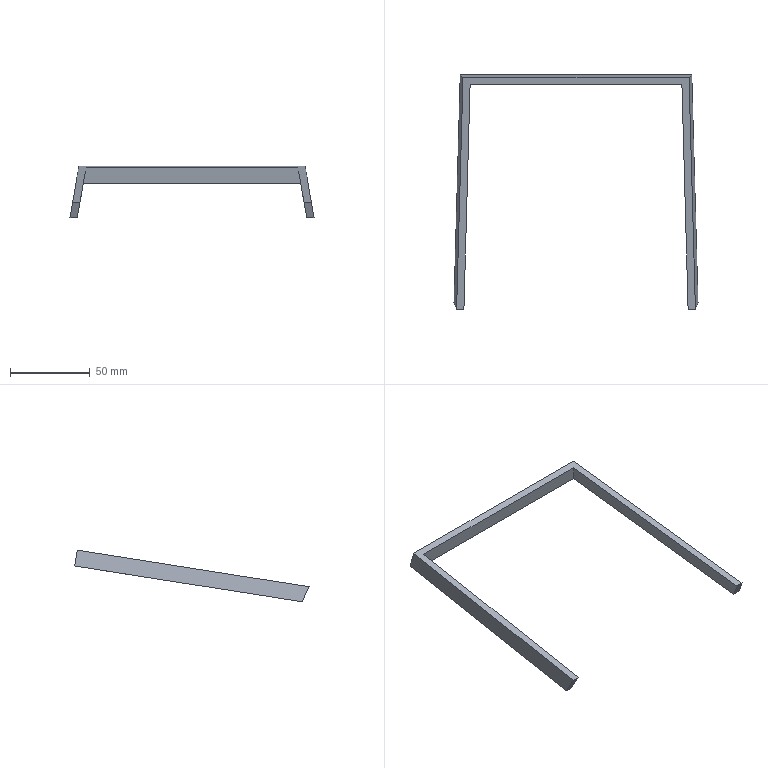Part | STEP file | 1-56.11 | 1 solid | 12 faces | box 152.783 x 146.73 x 32.367 mm | volume 19340 mm3 | plane 12
STEP:
#1=CARTESIAN_POINT('',(0.,0.,0.));
#2=DIRECTION('',(0.,0.,1.));
#3=DIRECTION('',(1.,0.,0.));
#4=AXIS2_PLACEMENT_3D('',#1,#2,#3);
#5=CARTESIAN_POINT('',(-71.823,28.822,-170.894));
#6=VERTEX_POINT('',#5);
#7=CARTESIAN_POINT('',(-76.391,28.822,-170.894));
#8=VERTEX_POINT('',#7);
#9=CARTESIAN_POINT('',(-71.823,28.822,-170.894));
#10=DIRECTION('',(-1.,0.,0.));
#11=VECTOR('',#10,1.);
#12=LINE('',#9,#11);
#13=CARTESIAN_POINT('',(-73.285,26.624,-166.179));
#14=DIRECTION('',(0.,0.9063,0.4226));
#15=DIRECTION('',(0.,0.4226,-0.9063));
#16=AXIS2_PLACEMENT_3D('',#13,#14,#15);
#17=PLANE('',#16);
#18=CARTESIAN_POINT('',(5.202,-1.462));
#19=DIRECTION('',(0.,1.));
#20=VECTOR('',#19,1.);
#21=LINE('',#18,#20);
#22=(GEOMETRIC_REPRESENTATION_CONTEXT(2)PARAMETRIC_REPRESENTATION_CONTEXT()REPRESENTATION_CONTEXT('',''));
#23=DEFINITIONAL_REPRESENTATION('',(#21),#22);
#24=PCURVE('',#17,#23);
#25=CARTESIAN_POINT('',(-72.146,100.013,-159.645));
#26=DIRECTION('',(0.,-0.1561,0.9877));
#27=DIRECTION('',(0.,0.9877,0.1561));
#28=AXIS2_PLACEMENT_3D('',#25,#26,#27);
#29=PLANE('',#28);
#30=CARTESIAN_POINT('',(-72.074,-0.3226));
#31=DIRECTION('',(0.,1.));
#32=VECTOR('',#31,1.);
#33=LINE('',#30,#32);
#34=(GEOMETRIC_REPRESENTATION_CONTEXT(2)PARAMETRIC_REPRESENTATION_CONTEXT()REPRESENTATION_CONTEXT('',''));
#35=DEFINITIONAL_REPRESENTATION('',(#33),#34);
#36=PCURVE('',#29,#35);
#37=SURFACE_CURVE('',#12,(#24,#36),.PCURVE_S1.);
#38=EDGE_CURVE('',#6,#8,#37,.T.);
#39=ORIENTED_EDGE('',*,*,#38,.T.);
#40=CARTESIAN_POINT('',(-74.747,24.425,-161.465));
#41=VERTEX_POINT('',#40);
#42=CARTESIAN_POINT('',(-76.391,28.822,-170.894));
#43=DIRECTION('',(0.1561,-0.4174,0.8952));
#44=VECTOR('',#43,1.);
#45=LINE('',#42,#44);
#46=CARTESIAN_POINT('',(5.202,3.106));
#47=DIRECTION('',(-0.9877,-0.1561));
#48=VECTOR('',#47,1.);
#49=LINE('',#46,#48);
#50=(GEOMETRIC_REPRESENTATION_CONTEXT(2)PARAMETRIC_REPRESENTATION_CONTEXT()REPRESENTATION_CONTEXT('',''));
#51=DEFINITIONAL_REPRESENTATION('',(#49),#50);
#52=PCURVE('',#17,#51);
#53=CARTESIAN_POINT('',(-63.833,90.,-98.893));
#54=DIRECTION('',(-0.9851,0.,0.1718));
#55=DIRECTION('',(0.1718,0.,0.9851));
#56=AXIS2_PLACEMENT_3D('',#53,#54,#55);
#57=PLANE('',#56);
#58=CARTESIAN_POINT('',(-73.088,-61.178));
#59=DIRECTION('',(0.9087,-0.4174));
#60=VECTOR('',#59,1.);
#61=LINE('',#58,#60);
#62=(GEOMETRIC_REPRESENTATION_CONTEXT(2)PARAMETRIC_REPRESENTATION_CONTEXT()REPRESENTATION_CONTEXT('',''));
#63=DEFINITIONAL_REPRESENTATION('',(#61),#62);
#64=PCURVE('',#57,#63);
#65=SURFACE_CURVE('',#45,(#52,#64),.PCURVE_S1.);
#66=EDGE_CURVE('',#8,#41,#65,.T.);
#67=ORIENTED_EDGE('',*,*,#66,.T.);
#68=CARTESIAN_POINT('',(-70.179,24.425,-161.465));
#69=VERTEX_POINT('',#68);
#70=CARTESIAN_POINT('',(-70.179,24.425,-161.465));
#71=DIRECTION('',(-1.,0.,0.));
#72=VECTOR('',#71,1.);
#73=LINE('',#70,#72);
#74=CARTESIAN_POINT('',(-5.202,-3.106));
#75=DIRECTION('',(0.,1.));
#76=VECTOR('',#75,1.);
#77=LINE('',#74,#76);
#78=(GEOMETRIC_REPRESENTATION_CONTEXT(2)PARAMETRIC_REPRESENTATION_CONTEXT()REPRESENTATION_CONTEXT('',''));
#79=DEFINITIONAL_REPRESENTATION('',(#77),#78);
#80=PCURVE('',#17,#79);
#81=CARTESIAN_POINT('',(-80.434,-353.244,-221.14));
#82=DIRECTION('',(0.,0.1561,-0.9877));
#83=DIRECTION('',(0.,-0.9877,-0.1561));
#84=AXIS2_PLACEMENT_3D('',#81,#82,#83);
#85=PLANE('',#84);
#86=CARTESIAN_POINT('',(-382.355,-10.256));
#87=DIRECTION('',(0.,1.));
#88=VECTOR('',#87,1.);
#89=LINE('',#86,#88);
#90=(GEOMETRIC_REPRESENTATION_CONTEXT(2)PARAMETRIC_REPRESENTATION_CONTEXT()REPRESENTATION_CONTEXT('',''));
#91=DEFINITIONAL_REPRESENTATION('',(#89),#90);
#92=PCURVE('',#85,#91);
#93=SURFACE_CURVE('',#73,(#80,#92),.PCURVE_S1.);
#94=EDGE_CURVE('',#69,#41,#93,.T.);
#95=ORIENTED_EDGE('',*,*,#94,.F.);
#96=CARTESIAN_POINT('',(-70.179,24.425,-161.465));
#97=DIRECTION('',(-0.1561,0.4174,-0.8952));
#98=VECTOR('',#97,1.);
#99=LINE('',#96,#98);
#100=CARTESIAN_POINT('',(-5.202,-3.106));
#101=DIRECTION('',(0.9877,0.1561));
#102=VECTOR('',#101,1.);
#103=LINE('',#100,#102);
#104=(GEOMETRIC_REPRESENTATION_CONTEXT(2)PARAMETRIC_REPRESENTATION_CONTEXT()REPRESENTATION_CONTEXT('',''));
#105=DEFINITIONAL_REPRESENTATION('',(#103),#104);
#106=PCURVE('',#17,#105);
#107=CARTESIAN_POINT('',(-59.4,90.,-99.667));
#108=DIRECTION('',(0.9851,0.,-0.1718));
#109=DIRECTION('',(-0.1718,0.,-0.9851));
#110=AXIS2_PLACEMENT_3D('',#107,#108,#109);
#111=PLANE('',#110);
#112=CARTESIAN_POINT('',(62.731,-65.575));
#113=DIRECTION('',(0.9087,0.4174));
#114=VECTOR('',#113,1.);
#115=LINE('',#112,#114);
#116=(GEOMETRIC_REPRESENTATION_CONTEXT(2)PARAMETRIC_REPRESENTATION_CONTEXT()REPRESENTATION_CONTEXT('',''));
#117=DEFINITIONAL_REPRESENTATION('',(#115),#116);
#118=PCURVE('',#111,#117);
#119=SURFACE_CURVE('',#99,(#106,#118),.PCURVE_S1.);
#120=EDGE_CURVE('',#69,#6,#119,.T.);
#121=ORIENTED_EDGE('',*,*,#120,.T.);
#122=EDGE_LOOP('',(#39,#67,#95,#121));
#123=FACE_BOUND('',#122,.F.);
#124=ADVANCED_FACE('',(#123),#17,.F.);
#125=ORIENTED_EDGE('',*,*,#120,.T.);
#126=CARTESIAN_POINT('',(-68.023,166.711,-149.107));
#127=VERTEX_POINT('',#126);
#128=CARTESIAN_POINT('',(-71.823,28.822,-170.894));
#129=DIRECTION('',(0.02721,0.9874,0.156));
#130=VECTOR('',#129,1.);
#131=LINE('',#128,#130);
#132=CARTESIAN_POINT('',(72.303,-61.178));
#133=DIRECTION('',(-0.1584,0.9874));
#134=VECTOR('',#133,1.);
#135=LINE('',#132,#134);
#136=(GEOMETRIC_REPRESENTATION_CONTEXT(2)PARAMETRIC_REPRESENTATION_CONTEXT()REPRESENTATION_CONTEXT('',''));
#137=DEFINITIONAL_REPRESENTATION('',(#135),#136);
#138=PCURVE('',#111,#137);
#139=CARTESIAN_POINT('',(-72.074,-0.3226));
#140=DIRECTION('',(0.9996,-0.02721));
#141=VECTOR('',#140,1.);
#142=LINE('',#139,#141);
#143=(GEOMETRIC_REPRESENTATION_CONTEXT(2)PARAMETRIC_REPRESENTATION_CONTEXT()REPRESENTATION_CONTEXT('',''));
#144=DEFINITIONAL_REPRESENTATION('',(#142),#143);
#145=PCURVE('',#29,#144);
#146=SURFACE_CURVE('',#131,(#138,#145),.PCURVE_S1.);
#147=EDGE_CURVE('',#6,#127,#146,.T.);
#148=ORIENTED_EDGE('',*,*,#147,.T.);
#149=CARTESIAN_POINT('',(-66.301,165.146,-139.231));
#150=VERTEX_POINT('',#149);
#151=CARTESIAN_POINT('',(-66.301,165.146,-139.231));
#152=DIRECTION('',(-0.1698,0.1542,-0.9733));
#153=VECTOR('',#152,1.);
#154=LINE('',#151,#153);
#155=CARTESIAN_POINT('',(40.162,75.146));
#156=DIRECTION('',(0.988,0.1542));
#157=VECTOR('',#156,1.);
#158=LINE('',#155,#157);
#159=(GEOMETRIC_REPRESENTATION_CONTEXT(2)PARAMETRIC_REPRESENTATION_CONTEXT()REPRESENTATION_CONTEXT('',''));
#160=DEFINITIONAL_REPRESENTATION('',(#158),#159);
#161=PCURVE('',#111,#160);
#162=CARTESIAN_POINT('',(0.,165.928,-144.17));
#163=DIRECTION('',(0.,0.9877,0.1565));
#164=DIRECTION('',(0.,0.1565,-0.9877));
#165=AXIS2_PLACEMENT_3D('',#162,#163,#164);
#166=PLANE('',#165);
#167=CARTESIAN_POINT('',(-5.,66.301));
#168=DIRECTION('',(0.9855,0.1698));
#169=VECTOR('',#168,1.);
#170=LINE('',#167,#169);
#171=(GEOMETRIC_REPRESENTATION_CONTEXT(2)PARAMETRIC_REPRESENTATION_CONTEXT()REPRESENTATION_CONTEXT('',''));
#172=DEFINITIONAL_REPRESENTATION('',(#170),#171);
#173=PCURVE('',#166,#172);
#174=SURFACE_CURVE('',#154,(#161,#173),.PCURVE_S1.);
#175=EDGE_CURVE('',#150,#127,#174,.T.);
#176=ORIENTED_EDGE('',*,*,#175,.F.);
#177=CARTESIAN_POINT('',(-66.3,165.146,-139.23));
#178=DIRECTION('',(-0.02721,-0.9874,-0.156));
#179=VECTOR('',#178,1.);
#180=LINE('',#177,#179);
#181=CARTESIAN_POINT('',(40.16,75.146));
#182=DIRECTION('',(0.1584,-0.9874));
#183=VECTOR('',#182,1.);
#184=LINE('',#181,#183);
#185=(GEOMETRIC_REPRESENTATION_CONTEXT(2)PARAMETRIC_REPRESENTATION_CONTEXT()REPRESENTATION_CONTEXT('',''));
#186=DEFINITIONAL_REPRESENTATION('',(#184),#185);
#187=PCURVE('',#111,#186);
#188=CARTESIAN_POINT('',(-524.821,-14.134));
#189=DIRECTION('',(0.9996,0.02721));
#190=VECTOR('',#189,1.);
#191=LINE('',#188,#190);
#192=(GEOMETRIC_REPRESENTATION_CONTEXT(2)PARAMETRIC_REPRESENTATION_CONTEXT()REPRESENTATION_CONTEXT('',''));
#193=DEFINITIONAL_REPRESENTATION('',(#191),#192);
#194=PCURVE('',#85,#193);
#195=SURFACE_CURVE('',#180,(#187,#194),.PCURVE_S1.);
#196=EDGE_CURVE('',#150,#69,#195,.T.);
#197=ORIENTED_EDGE('',*,*,#196,.T.);
#198=EDGE_LOOP('',(#125,#148,#176,#197));
#199=FACE_BOUND('',#198,.T.);
#200=ADVANCED_FACE('',(#199),#111,.T.);
#201=ORIENTED_EDGE('',*,*,#175,.F.);
#202=CARTESIAN_POINT('',(66.301,165.146,-139.231));
#203=VERTEX_POINT('',#202);
#204=CARTESIAN_POINT('',(66.301,165.146,-139.231));
#205=DIRECTION('',(-1.,0.,0.));
#206=VECTOR('',#205,1.);
#207=LINE('',#204,#206);
#208=CARTESIAN_POINT('',(-5.,-66.301));
#209=DIRECTION('',(0.,1.));
#210=VECTOR('',#209,1.);
#211=LINE('',#208,#210);
#212=(GEOMETRIC_REPRESENTATION_CONTEXT(2)PARAMETRIC_REPRESENTATION_CONTEXT()REPRESENTATION_CONTEXT('',''));
#213=DEFINITIONAL_REPRESENTATION('',(#211),#212);
#214=PCURVE('',#166,#213);
#215=CARTESIAN_POINT('',(-524.822,-146.735));
#216=DIRECTION('',(0.,1.));
#217=VECTOR('',#216,1.);
#218=LINE('',#215,#217);
#219=(GEOMETRIC_REPRESENTATION_CONTEXT(2)PARAMETRIC_REPRESENTATION_CONTEXT()REPRESENTATION_CONTEXT('',''));
#220=DEFINITIONAL_REPRESENTATION('',(#218),#219);
#221=PCURVE('',#85,#220);
#222=SURFACE_CURVE('',#207,(#214,#221),.PCURVE_S1.);
#223=EDGE_CURVE('',#203,#150,#222,.T.);
#224=ORIENTED_EDGE('',*,*,#223,.F.);
#225=CARTESIAN_POINT('',(68.023,166.711,-149.107));
#226=VERTEX_POINT('',#225);
#227=CARTESIAN_POINT('',(66.301,165.146,-139.231));
#228=DIRECTION('',(0.1698,0.1542,-0.9733));
#229=VECTOR('',#228,1.);
#230=LINE('',#227,#229);
#231=CARTESIAN_POINT('',(-5.,-66.301));
#232=DIRECTION('',(0.9855,-0.1698));
#233=VECTOR('',#232,1.);
#234=LINE('',#231,#233);
#235=(GEOMETRIC_REPRESENTATION_CONTEXT(2)PARAMETRIC_REPRESENTATION_CONTEXT()REPRESENTATION_CONTEXT('',''));
#236=DEFINITIONAL_REPRESENTATION('',(#234),#235);
#237=PCURVE('',#166,#236);
#238=CARTESIAN_POINT('',(59.4,90.,-99.667));
#239=DIRECTION('',(-0.9851,0.,-0.1718));
#240=DIRECTION('',(-0.1718,0.,0.9851));
#241=AXIS2_PLACEMENT_3D('',#238,#239,#240);
#242=PLANE('',#241);
#243=CARTESIAN_POINT('',(-40.162,75.146));
#244=DIRECTION('',(-0.988,0.1542));
#245=VECTOR('',#244,1.);
#246=LINE('',#243,#245);
#247=(GEOMETRIC_REPRESENTATION_CONTEXT(2)PARAMETRIC_REPRESENTATION_CONTEXT()REPRESENTATION_CONTEXT('',''));
#248=DEFINITIONAL_REPRESENTATION('',(#246),#247);
#249=PCURVE('',#242,#248);
#250=SURFACE_CURVE('',#230,(#237,#249),.PCURVE_S1.);
#251=EDGE_CURVE('',#203,#226,#250,.T.);
#252=ORIENTED_EDGE('',*,*,#251,.T.);
#253=CARTESIAN_POINT('',(68.023,166.711,-149.108));
#254=DIRECTION('',(-1.,0.,0.));
#255=VECTOR('',#254,1.);
#256=LINE('',#253,#255);
#257=CARTESIAN_POINT('',(5.,-68.023));
#258=DIRECTION('',(0.,1.));
#259=VECTOR('',#258,1.);
#260=LINE('',#257,#259);
#261=(GEOMETRIC_REPRESENTATION_CONTEXT(2)PARAMETRIC_REPRESENTATION_CONTEXT()REPRESENTATION_CONTEXT('',''));
#262=DEFINITIONAL_REPRESENTATION('',(#260),#261);
#263=PCURVE('',#166,#262);
#264=CARTESIAN_POINT('',(43.297,126.169,-155.531));
#265=DIRECTION('',(0.,-0.1565,0.9877));
#266=DIRECTION('',(0.,0.9877,0.1565));
#267=AXIS2_PLACEMENT_3D('',#264,#265,#266);
#268=PLANE('',#267);
#269=CARTESIAN_POINT('',(41.047,-24.726));
#270=DIRECTION('',(0.,1.));
#271=VECTOR('',#270,1.);
#272=LINE('',#269,#271);
#273=(GEOMETRIC_REPRESENTATION_CONTEXT(2)PARAMETRIC_REPRESENTATION_CONTEXT()REPRESENTATION_CONTEXT('',''));
#274=DEFINITIONAL_REPRESENTATION('',(#272),#273);
#275=PCURVE('',#268,#274);
#276=SURFACE_CURVE('',#256,(#263,#275),.PCURVE_S1.);
#277=EDGE_CURVE('',#226,#127,#276,.T.);
#278=ORIENTED_EDGE('',*,*,#277,.T.);
#279=EDGE_LOOP('',(#201,#224,#252,#278));
#280=FACE_BOUND('',#279,.F.);
#281=ADVANCED_FACE('',(#280),#166,.F.);
#282=CARTESIAN_POINT('',(71.823,28.822,-170.894));
#283=VERTEX_POINT('',#282);
#284=CARTESIAN_POINT('',(70.179,24.425,-161.465));
#285=VERTEX_POINT('',#284);
#286=CARTESIAN_POINT('',(71.823,28.822,-170.894));
#287=DIRECTION('',(-0.1561,-0.4174,0.8952));
#288=VECTOR('',#287,1.);
#289=LINE('',#286,#288);
#290=CARTESIAN_POINT('',(-72.303,-61.178));
#291=DIRECTION('',(0.9087,-0.4174));
#292=VECTOR('',#291,1.);
#293=LINE('',#290,#292);
#294=(GEOMETRIC_REPRESENTATION_CONTEXT(2)PARAMETRIC_REPRESENTATION_CONTEXT()REPRESENTATION_CONTEXT('',''));
#295=DEFINITIONAL_REPRESENTATION('',(#293),#294);
#296=PCURVE('',#242,#295);
#297=CARTESIAN_POINT('',(73.285,26.624,-166.179));
#298=DIRECTION('',(0.,0.9063,0.4226));
#299=DIRECTION('',(0.,0.4226,-0.9063));
#300=AXIS2_PLACEMENT_3D('',#297,#298,#299);
#301=PLANE('',#300);
#302=CARTESIAN_POINT('',(5.202,1.462));
#303=DIRECTION('',(-0.9877,0.1561));
#304=VECTOR('',#303,1.);
#305=LINE('',#302,#304);
#306=(GEOMETRIC_REPRESENTATION_CONTEXT(2)PARAMETRIC_REPRESENTATION_CONTEXT()REPRESENTATION_CONTEXT('',''));
#307=DEFINITIONAL_REPRESENTATION('',(#305),#306);
#308=PCURVE('',#301,#307);
#309=SURFACE_CURVE('',#289,(#296,#308),.PCURVE_S1.);
#310=EDGE_CURVE('',#283,#285,#309,.T.);
#311=ORIENTED_EDGE('',*,*,#310,.T.);
#312=CARTESIAN_POINT('',(70.179,24.425,-161.465));
#313=DIRECTION('',(-0.02721,0.9874,0.156));
#314=VECTOR('',#313,1.);
#315=LINE('',#312,#314);
#316=CARTESIAN_POINT('',(-62.731,-65.575));
#317=DIRECTION('',(0.1584,0.9874));
#318=VECTOR('',#317,1.);
#319=LINE('',#316,#318);
#320=(GEOMETRIC_REPRESENTATION_CONTEXT(2)PARAMETRIC_REPRESENTATION_CONTEXT()REPRESENTATION_CONTEXT('',''));
#321=DEFINITIONAL_REPRESENTATION('',(#319),#320);
#322=PCURVE('',#242,#321);
#323=CARTESIAN_POINT('',(-382.355,-150.613));
#324=DIRECTION('',(-0.9996,0.02721));
#325=VECTOR('',#324,1.);
#326=LINE('',#323,#325);
#327=(GEOMETRIC_REPRESENTATION_CONTEXT(2)PARAMETRIC_REPRESENTATION_CONTEXT()REPRESENTATION_CONTEXT('',''));
#328=DEFINITIONAL_REPRESENTATION('',(#326),#327);
#329=PCURVE('',#85,#328);
#330=SURFACE_CURVE('',#315,(#322,#329),.PCURVE_S1.);
#331=EDGE_CURVE('',#285,#203,#330,.T.);
#332=ORIENTED_EDGE('',*,*,#331,.T.);
#333=ORIENTED_EDGE('',*,*,#251,.T.);
#334=CARTESIAN_POINT('',(68.023,166.711,-149.106));
#335=DIRECTION('',(0.02721,-0.9874,-0.156));
#336=VECTOR('',#335,1.);
#337=LINE('',#334,#336);
#338=CARTESIAN_POINT('',(-50.186,76.711));
#339=DIRECTION('',(-0.1584,-0.9874));
#340=VECTOR('',#339,1.);
#341=LINE('',#338,#340);
#342=(GEOMETRIC_REPRESENTATION_CONTEXT(2)PARAMETRIC_REPRESENTATION_CONTEXT()REPRESENTATION_CONTEXT('',''));
#343=DEFINITIONAL_REPRESENTATION('',(#341),#342);
#344=PCURVE('',#242,#343);
#345=CARTESIAN_POINT('',(72.146,99.989,-159.649));
#346=DIRECTION('',(0.,-0.1561,0.9877));
#347=DIRECTION('',(0.,0.9877,0.1561));
#348=AXIS2_PLACEMENT_3D('',#345,#346,#347);
#349=PLANE('',#348);
#350=CARTESIAN_POINT('',(67.549,4.123));
#351=DIRECTION('',(-0.9996,-0.02721));
#352=VECTOR('',#351,1.);
#353=LINE('',#350,#352);
#354=(GEOMETRIC_REPRESENTATION_CONTEXT(2)PARAMETRIC_REPRESENTATION_CONTEXT()REPRESENTATION_CONTEXT('',''));
#355=DEFINITIONAL_REPRESENTATION('',(#353),#354);
#356=PCURVE('',#349,#355);
#357=SURFACE_CURVE('',#337,(#344,#356),.PCURVE_S1.);
#358=EDGE_CURVE('',#226,#283,#357,.T.);
#359=ORIENTED_EDGE('',*,*,#358,.T.);
#360=EDGE_LOOP('',(#311,#332,#333,#359));
#361=FACE_BOUND('',#360,.T.);
#362=ADVANCED_FACE('',(#361),#242,.T.);
#363=CARTESIAN_POINT('',(76.391,28.822,-170.894));
#364=VERTEX_POINT('',#363);
#365=CARTESIAN_POINT('',(76.391,28.822,-170.894));
#366=DIRECTION('',(-1.,0.,0.));
#367=VECTOR('',#366,1.);
#368=LINE('',#365,#367);
#369=CARTESIAN_POINT('',(-72.05,-4.245));
#370=DIRECTION('',(0.,1.));
#371=VECTOR('',#370,1.);
#372=LINE('',#369,#371);
#373=(GEOMETRIC_REPRESENTATION_CONTEXT(2)PARAMETRIC_REPRESENTATION_CONTEXT()REPRESENTATION_CONTEXT('',''));
#374=DEFINITIONAL_REPRESENTATION('',(#372),#373);
#375=PCURVE('',#349,#374);
#376=CARTESIAN_POINT('',(5.202,-3.106));
#377=DIRECTION('',(0.,1.));
#378=VECTOR('',#377,1.);
#379=LINE('',#376,#378);
#380=(GEOMETRIC_REPRESENTATION_CONTEXT(2)PARAMETRIC_REPRESENTATION_CONTEXT()REPRESENTATION_CONTEXT('',''));
#381=DEFINITIONAL_REPRESENTATION('',(#379),#380);
#382=PCURVE('',#301,#381);
#383=SURFACE_CURVE('',#368,(#375,#382),.PCURVE_S1.);
#384=EDGE_CURVE('',#364,#283,#383,.T.);
#385=ORIENTED_EDGE('',*,*,#384,.F.);
#386=CARTESIAN_POINT('',(72.591,166.711,-149.107));
#387=VERTEX_POINT('',#386);
#388=CARTESIAN_POINT('',(76.391,28.822,-170.894));
#389=DIRECTION('',(-0.02721,0.9874,0.156));
#390=VECTOR('',#389,1.);
#391=LINE('',#388,#390);
#392=CARTESIAN_POINT('',(-72.05,-4.245));
#393=DIRECTION('',(0.9996,0.02721));
#394=VECTOR('',#393,1.);
#395=LINE('',#392,#394);
#396=(GEOMETRIC_REPRESENTATION_CONTEXT(2)PARAMETRIC_REPRESENTATION_CONTEXT()REPRESENTATION_CONTEXT('',''));
#397=DEFINITIONAL_REPRESENTATION('',(#395),#396);
#398=PCURVE('',#349,#397);
#399=CARTESIAN_POINT('',(63.833,90.,-98.893));
#400=DIRECTION('',(0.9851,0.,0.1718));
#401=DIRECTION('',(0.1718,0.,-0.9851));
#402=AXIS2_PLACEMENT_3D('',#399,#400,#401);
#403=PLANE('',#402);
#404=CARTESIAN_POINT('',(73.088,-61.178));
#405=DIRECTION('',(-0.1584,0.9874));
#406=VECTOR('',#405,1.);
#407=LINE('',#404,#406);
#408=(GEOMETRIC_REPRESENTATION_CONTEXT(2)PARAMETRIC_REPRESENTATION_CONTEXT()REPRESENTATION_CONTEXT('',''));
#409=DEFINITIONAL_REPRESENTATION('',(#407),#408);
#410=PCURVE('',#403,#409);
#411=SURFACE_CURVE('',#391,(#398,#410),.PCURVE_S1.);
#412=EDGE_CURVE('',#364,#387,#411,.T.);
#413=ORIENTED_EDGE('',*,*,#412,.T.);
#414=CARTESIAN_POINT('',(72.591,166.711,-149.108));
#415=DIRECTION('',(-1.,0.,0.));
#416=VECTOR('',#415,1.);
#417=LINE('',#414,#416);
#418=CARTESIAN_POINT('',(67.55,-0.4453));
#419=DIRECTION('',(0.,1.));
#420=VECTOR('',#419,1.);
#421=LINE('',#418,#420);
#422=(GEOMETRIC_REPRESENTATION_CONTEXT(2)PARAMETRIC_REPRESENTATION_CONTEXT()REPRESENTATION_CONTEXT('',''));
#423=DEFINITIONAL_REPRESENTATION('',(#421),#422);
#424=PCURVE('',#349,#423);
#425=CARTESIAN_POINT('',(41.047,-29.294));
#426=DIRECTION('',(0.,1.));
#427=VECTOR('',#426,1.);
#428=LINE('',#425,#427);
#429=(GEOMETRIC_REPRESENTATION_CONTEXT(2)PARAMETRIC_REPRESENTATION_CONTEXT()REPRESENTATION_CONTEXT('',''));
#430=DEFINITIONAL_REPRESENTATION('',(#428),#429);
#431=PCURVE('',#268,#430);
#432=SURFACE_CURVE('',#417,(#424,#431),.PCURVE_S1.);
#433=EDGE_CURVE('',#387,#226,#432,.T.);
#434=ORIENTED_EDGE('',*,*,#433,.T.);
#435=ORIENTED_EDGE('',*,*,#358,.T.);
#436=EDGE_LOOP('',(#385,#413,#434,#435));
#437=FACE_BOUND('',#436,.F.);
#438=ADVANCED_FACE('',(#437),#349,.F.);
#439=ORIENTED_EDGE('',*,*,#384,.T.);
#440=ORIENTED_EDGE('',*,*,#310,.T.);
#441=CARTESIAN_POINT('',(74.747,24.425,-161.465));
#442=VERTEX_POINT('',#441);
#443=CARTESIAN_POINT('',(74.747,24.425,-161.465));
#444=DIRECTION('',(-1.,0.,0.));
#445=VECTOR('',#444,1.);
#446=LINE('',#443,#445);
#447=CARTESIAN_POINT('',(-5.202,-1.462));
#448=DIRECTION('',(0.,1.));
#449=VECTOR('',#448,1.);
#450=LINE('',#447,#449);
#451=(GEOMETRIC_REPRESENTATION_CONTEXT(2)PARAMETRIC_REPRESENTATION_CONTEXT()REPRESENTATION_CONTEXT('',''));
#452=DEFINITIONAL_REPRESENTATION('',(#450),#451);
#453=PCURVE('',#301,#452);
#454=CARTESIAN_POINT('',(-382.355,-155.181));
#455=DIRECTION('',(0.,1.));
#456=VECTOR('',#455,1.);
#457=LINE('',#454,#456);
#458=(GEOMETRIC_REPRESENTATION_CONTEXT(2)PARAMETRIC_REPRESENTATION_CONTEXT()REPRESENTATION_CONTEXT('',''));
#459=DEFINITIONAL_REPRESENTATION('',(#457),#458);
#460=PCURVE('',#85,#459);
#461=SURFACE_CURVE('',#446,(#453,#460),.PCURVE_S1.);
#462=EDGE_CURVE('',#442,#285,#461,.T.);
#463=ORIENTED_EDGE('',*,*,#462,.F.);
#464=CARTESIAN_POINT('',(74.747,24.425,-161.465));
#465=DIRECTION('',(0.1561,0.4174,-0.8952));
#466=VECTOR('',#465,1.);
#467=LINE('',#464,#466);
#468=CARTESIAN_POINT('',(-5.202,-1.462));
#469=DIRECTION('',(0.9877,-0.1561));
#470=VECTOR('',#469,1.);
#471=LINE('',#468,#470);
#472=(GEOMETRIC_REPRESENTATION_CONTEXT(2)PARAMETRIC_REPRESENTATION_CONTEXT()REPRESENTATION_CONTEXT('',''));
#473=DEFINITIONAL_REPRESENTATION('',(#471),#472);
#474=PCURVE('',#301,#473);
#475=CARTESIAN_POINT('',(63.516,-65.575));
#476=DIRECTION('',(0.9087,0.4174));
#477=VECTOR('',#476,1.);
#478=LINE('',#475,#477);
#479=(GEOMETRIC_REPRESENTATION_CONTEXT(2)PARAMETRIC_REPRESENTATION_CONTEXT()REPRESENTATION_CONTEXT('',''));
#480=DEFINITIONAL_REPRESENTATION('',(#478),#479);
#481=PCURVE('',#403,#480);
#482=SURFACE_CURVE('',#467,(#474,#481),.PCURVE_S1.);
#483=EDGE_CURVE('',#442,#364,#482,.T.);
#484=ORIENTED_EDGE('',*,*,#483,.T.);
#485=EDGE_LOOP('',(#439,#440,#463,#484));
#486=FACE_BOUND('',#485,.F.);
#487=ADVANCED_FACE('',(#486),#301,.F.);
#488=ORIENTED_EDGE('',*,*,#66,.T.);
#489=CARTESIAN_POINT('',(-70.746,169.591,-138.527));
#490=VERTEX_POINT('',#489);
#491=CARTESIAN_POINT('',(-74.747,24.425,-161.465));
#492=DIRECTION('',(0.02721,0.9874,0.156));
#493=VECTOR('',#492,1.);
#494=LINE('',#491,#493);
#495=CARTESIAN_POINT('',(-63.516,-65.575));
#496=DIRECTION('',(0.1584,0.9874));
#497=VECTOR('',#496,1.);
#498=LINE('',#495,#497);
#499=(GEOMETRIC_REPRESENTATION_CONTEXT(2)PARAMETRIC_REPRESENTATION_CONTEXT()REPRESENTATION_CONTEXT('',''));
#500=DEFINITIONAL_REPRESENTATION('',(#498),#499);
#501=PCURVE('',#57,#500);
#502=CARTESIAN_POINT('',(-382.355,-5.688));
#503=DIRECTION('',(-0.9996,-0.02721));
#504=VECTOR('',#503,1.);
#505=LINE('',#502,#504);
#506=(GEOMETRIC_REPRESENTATION_CONTEXT(2)PARAMETRIC_REPRESENTATION_CONTEXT()REPRESENTATION_CONTEXT('',''));
#507=DEFINITIONAL_REPRESENTATION('',(#505),#506);
#508=PCURVE('',#85,#507);
#509=SURFACE_CURVE('',#494,(#501,#508),.PCURVE_S1.);
#510=EDGE_CURVE('',#41,#490,#509,.T.);
#511=ORIENTED_EDGE('',*,*,#510,.T.);
#512=CARTESIAN_POINT('',(-72.469,171.155,-148.404));
#513=VERTEX_POINT('',#512);
#514=CARTESIAN_POINT('',(-70.746,169.591,-138.527));
#515=DIRECTION('',(-0.1698,0.1542,-0.9733));
#516=VECTOR('',#515,1.);
#517=LINE('',#514,#516);
#518=CARTESIAN_POINT('',(-40.232,79.591));
#519=DIRECTION('',(-0.988,0.1542));
#520=VECTOR('',#519,1.);
#521=LINE('',#518,#520);
#522=(GEOMETRIC_REPRESENTATION_CONTEXT(2)PARAMETRIC_REPRESENTATION_CONTEXT()REPRESENTATION_CONTEXT('',''));
#523=DEFINITIONAL_REPRESENTATION('',(#521),#522);
#524=PCURVE('',#57,#523);
#525=CARTESIAN_POINT('',(-50.881,178.335,-193.72));
#526=DIRECTION('',(0.,-0.9877,-0.1565));
#527=DIRECTION('',(0.,-0.1565,0.9877));
#528=AXIS2_PLACEMENT_3D('',#525,#526,#527);
#529=PLANE('',#528);
#530=CARTESIAN_POINT('',(55.881,19.865));
#531=DIRECTION('',(-0.9855,0.1698));
#532=VECTOR('',#531,1.);
#533=LINE('',#530,#532);
#534=(GEOMETRIC_REPRESENTATION_CONTEXT(2)PARAMETRIC_REPRESENTATION_CONTEXT()REPRESENTATION_CONTEXT('',''));
#535=DEFINITIONAL_REPRESENTATION('',(#533),#534);
#536=PCURVE('',#529,#535);
#537=SURFACE_CURVE('',#517,(#524,#536),.PCURVE_S1.);
#538=EDGE_CURVE('',#490,#513,#537,.T.);
#539=ORIENTED_EDGE('',*,*,#538,.T.);
#540=CARTESIAN_POINT('',(-76.391,28.822,-170.894));
#541=DIRECTION('',(0.02721,0.9874,0.156));
#542=VECTOR('',#541,1.);
#543=LINE('',#540,#542);
#544=CARTESIAN_POINT('',(-73.088,-61.178));
#545=DIRECTION('',(0.1584,0.9874));
#546=VECTOR('',#545,1.);
#547=LINE('',#544,#546);
#548=(GEOMETRIC_REPRESENTATION_CONTEXT(2)PARAMETRIC_REPRESENTATION_CONTEXT()REPRESENTATION_CONTEXT('',''));
#549=DEFINITIONAL_REPRESENTATION('',(#547),#548);
#550=PCURVE('',#57,#549);
#551=CARTESIAN_POINT('',(-72.074,4.245));
#552=DIRECTION('',(0.9996,-0.02721));
#553=VECTOR('',#552,1.);
#554=LINE('',#551,#553);
#555=(GEOMETRIC_REPRESENTATION_CONTEXT(2)PARAMETRIC_REPRESENTATION_CONTEXT()REPRESENTATION_CONTEXT('',''));
#556=DEFINITIONAL_REPRESENTATION('',(#554),#555);
#557=PCURVE('',#29,#556);
#558=SURFACE_CURVE('',#543,(#550,#557),.PCURVE_S1.);
#559=EDGE_CURVE('',#8,#513,#558,.T.);
#560=ORIENTED_EDGE('',*,*,#559,.F.);
#561=EDGE_LOOP('',(#488,#511,#539,#560));
#562=FACE_BOUND('',#561,.T.);
#563=ADVANCED_FACE('',(#562),#57,.T.);
#564=ORIENTED_EDGE('',*,*,#38,.F.);
#565=ORIENTED_EDGE('',*,*,#147,.T.);
#566=CARTESIAN_POINT('',(-67.901,171.155,-148.404));
#567=VERTEX_POINT('',#566);
#568=CARTESIAN_POINT('',(-68.023,166.711,-149.106));
#569=DIRECTION('',(0.02721,0.9874,0.156));
#570=VECTOR('',#569,1.);
#571=LINE('',#568,#570);
#572=CARTESIAN_POINT('',(67.525,-4.123));
#573=DIRECTION('',(0.9996,-0.02721));
#574=VECTOR('',#573,1.);
#575=LINE('',#572,#574);
#576=(GEOMETRIC_REPRESENTATION_CONTEXT(2)PARAMETRIC_REPRESENTATION_CONTEXT()REPRESENTATION_CONTEXT('',''));
#577=DEFINITIONAL_REPRESENTATION('',(#575),#576);
#578=PCURVE('',#29,#577);
#579=CARTESIAN_POINT('',(41.047,111.32));
#580=DIRECTION('',(0.9996,-0.02721));
#581=VECTOR('',#580,1.);
#582=LINE('',#579,#581);
#583=(GEOMETRIC_REPRESENTATION_CONTEXT(2)PARAMETRIC_REPRESENTATION_CONTEXT()REPRESENTATION_CONTEXT('',''));
#584=DEFINITIONAL_REPRESENTATION('',(#582),#583);
#585=PCURVE('',#268,#584);
#586=SURFACE_CURVE('',#571,(#578,#585),.PCURVE_S1.);
#587=EDGE_CURVE('',#127,#567,#586,.T.);
#588=ORIENTED_EDGE('',*,*,#587,.T.);
#589=CARTESIAN_POINT('',(-67.901,171.155,-148.404));
#590=DIRECTION('',(-1.,0.,0.));
#591=VECTOR('',#590,1.);
#592=LINE('',#589,#591);
#593=CARTESIAN_POINT('',(72.025,-4.245));
#594=DIRECTION('',(0.,1.));
#595=VECTOR('',#594,1.);
#596=LINE('',#593,#595);
#597=(GEOMETRIC_REPRESENTATION_CONTEXT(2)PARAMETRIC_REPRESENTATION_CONTEXT()REPRESENTATION_CONTEXT('',''));
#598=DEFINITIONAL_REPRESENTATION('',(#596),#597);
#599=PCURVE('',#29,#598);
#600=CARTESIAN_POINT('',(45.881,17.019));
#601=DIRECTION('',(0.,1.));
#602=VECTOR('',#601,1.);
#603=LINE('',#600,#602);
#604=(GEOMETRIC_REPRESENTATION_CONTEXT(2)PARAMETRIC_REPRESENTATION_CONTEXT()REPRESENTATION_CONTEXT('',''));
#605=DEFINITIONAL_REPRESENTATION('',(#603),#604);
#606=PCURVE('',#529,#605);
#607=SURFACE_CURVE('',#592,(#599,#606),.PCURVE_S1.);
#608=EDGE_CURVE('',#567,#513,#607,.T.);
#609=ORIENTED_EDGE('',*,*,#608,.T.);
#610=ORIENTED_EDGE('',*,*,#559,.F.);
#611=EDGE_LOOP('',(#564,#565,#588,#609,#610));
#612=FACE_BOUND('',#611,.F.);
#613=ADVANCED_FACE('',(#612),#29,.F.);
#614=ORIENTED_EDGE('',*,*,#433,.F.);
#615=CARTESIAN_POINT('',(72.469,171.155,-148.404));
#616=VERTEX_POINT('',#615);
#617=CARTESIAN_POINT('',(72.469,171.155,-148.404));
#618=DIRECTION('',(0.02728,-0.9873,-0.1564));
#619=VECTOR('',#618,1.);
#620=LINE('',#617,#619);
#621=CARTESIAN_POINT('',(45.547,-29.171));
#622=DIRECTION('',(-0.9996,-0.02728));
#623=VECTOR('',#622,1.);
#624=LINE('',#621,#623);
#625=(GEOMETRIC_REPRESENTATION_CONTEXT(2)PARAMETRIC_REPRESENTATION_CONTEXT()REPRESENTATION_CONTEXT('',''));
#626=DEFINITIONAL_REPRESENTATION('',(#624),#625);
#627=PCURVE('',#268,#626);
#628=CARTESIAN_POINT('',(50.258,81.155));
#629=DIRECTION('',(0.1588,-0.9873));
#630=VECTOR('',#629,1.);
#631=LINE('',#628,#630);
#632=(GEOMETRIC_REPRESENTATION_CONTEXT(2)PARAMETRIC_REPRESENTATION_CONTEXT()REPRESENTATION_CONTEXT('',''));
#633=DEFINITIONAL_REPRESENTATION('',(#631),#632);
#634=PCURVE('',#403,#633);
#635=SURFACE_CURVE('',#620,(#627,#634),.PCURVE_S1.);
#636=EDGE_CURVE('',#616,#387,#635,.T.);
#637=ORIENTED_EDGE('',*,*,#636,.F.);
#638=CARTESIAN_POINT('',(72.469,171.155,-148.404));
#639=DIRECTION('',(-1.,0.,0.));
#640=VECTOR('',#639,1.);
#641=LINE('',#638,#640);
#642=CARTESIAN_POINT('',(45.547,-29.171));
#643=DIRECTION('',(0.,1.));
#644=VECTOR('',#643,1.);
#645=LINE('',#642,#644);
#646=(GEOMETRIC_REPRESENTATION_CONTEXT(2)PARAMETRIC_REPRESENTATION_CONTEXT()REPRESENTATION_CONTEXT('',''));
#647=DEFINITIONAL_REPRESENTATION('',(#645),#646);
#648=PCURVE('',#268,#647);
#649=CARTESIAN_POINT('',(45.881,-123.35));
#650=DIRECTION('',(0.,1.));
#651=VECTOR('',#650,1.);
#652=LINE('',#649,#651);
#653=(GEOMETRIC_REPRESENTATION_CONTEXT(2)PARAMETRIC_REPRESENTATION_CONTEXT()REPRESENTATION_CONTEXT('',''));
#654=DEFINITIONAL_REPRESENTATION('',(#652),#653);
#655=PCURVE('',#529,#654);
#656=SURFACE_CURVE('',#641,(#648,#655),.PCURVE_S1.);
#657=EDGE_CURVE('',#616,#567,#656,.T.);
#658=ORIENTED_EDGE('',*,*,#657,.T.);
#659=ORIENTED_EDGE('',*,*,#587,.F.);
#660=ORIENTED_EDGE('',*,*,#277,.F.);
#661=EDGE_LOOP('',(#614,#637,#658,#659,#660));
#662=FACE_BOUND('',#661,.F.);
#663=ADVANCED_FACE('',(#662),#268,.F.);
#664=ORIENTED_EDGE('',*,*,#483,.T.);
#665=ORIENTED_EDGE('',*,*,#412,.T.);
#666=ORIENTED_EDGE('',*,*,#636,.F.);
#667=CARTESIAN_POINT('',(70.746,169.591,-138.527));
#668=VERTEX_POINT('',#667);
#669=CARTESIAN_POINT('',(72.469,171.155,-148.404));
#670=DIRECTION('',(-0.1698,-0.1542,0.9733));
#671=VECTOR('',#670,1.);
#672=LINE('',#669,#671);
#673=CARTESIAN_POINT('',(50.258,81.155));
#674=DIRECTION('',(-0.988,-0.1542));
#675=VECTOR('',#674,1.);
#676=LINE('',#673,#675);
#677=(GEOMETRIC_REPRESENTATION_CONTEXT(2)PARAMETRIC_REPRESENTATION_CONTEXT()REPRESENTATION_CONTEXT('',''));
#678=DEFINITIONAL_REPRESENTATION('',(#676),#677);
#679=PCURVE('',#403,#678);
#680=CARTESIAN_POINT('',(45.881,-123.35));
#681=DIRECTION('',(0.9855,0.1698));
#682=VECTOR('',#681,1.);
#683=LINE('',#680,#682);
#684=(GEOMETRIC_REPRESENTATION_CONTEXT(2)PARAMETRIC_REPRESENTATION_CONTEXT()REPRESENTATION_CONTEXT('',''));
#685=DEFINITIONAL_REPRESENTATION('',(#683),#684);
#686=PCURVE('',#529,#685);
#687=SURFACE_CURVE('',#672,(#679,#686),.PCURVE_S1.);
#688=EDGE_CURVE('',#616,#668,#687,.T.);
#689=ORIENTED_EDGE('',*,*,#688,.T.);
#690=CARTESIAN_POINT('',(74.747,24.425,-161.465));
#691=DIRECTION('',(-0.02721,0.9874,0.156));
#692=VECTOR('',#691,1.);
#693=LINE('',#690,#692);
#694=CARTESIAN_POINT('',(63.516,-65.575));
#695=DIRECTION('',(-0.1584,0.9874));
#696=VECTOR('',#695,1.);
#697=LINE('',#694,#696);
#698=(GEOMETRIC_REPRESENTATION_CONTEXT(2)PARAMETRIC_REPRESENTATION_CONTEXT()REPRESENTATION_CONTEXT('',''));
#699=DEFINITIONAL_REPRESENTATION('',(#697),#698);
#700=PCURVE('',#403,#699);
#701=CARTESIAN_POINT('',(-382.355,-155.181));
#702=DIRECTION('',(-0.9996,0.02721));
#703=VECTOR('',#702,1.);
#704=LINE('',#701,#703);
#705=(GEOMETRIC_REPRESENTATION_CONTEXT(2)PARAMETRIC_REPRESENTATION_CONTEXT()REPRESENTATION_CONTEXT('',''));
#706=DEFINITIONAL_REPRESENTATION('',(#704),#705);
#707=PCURVE('',#85,#706);
#708=SURFACE_CURVE('',#693,(#700,#707),.PCURVE_S1.);
#709=EDGE_CURVE('',#442,#668,#708,.T.);
#710=ORIENTED_EDGE('',*,*,#709,.F.);
#711=EDGE_LOOP('',(#664,#665,#666,#689,#710));
#712=FACE_BOUND('',#711,.T.);
#713=ADVANCED_FACE('',(#712),#403,.T.);
#714=ORIENTED_EDGE('',*,*,#538,.T.);
#715=ORIENTED_EDGE('',*,*,#608,.F.);
#716=ORIENTED_EDGE('',*,*,#657,.F.);
#717=ORIENTED_EDGE('',*,*,#688,.T.);
#718=CARTESIAN_POINT('',(70.746,169.591,-138.527));
#719=DIRECTION('',(-1.,0.,0.));
#720=VECTOR('',#719,1.);
#721=LINE('',#718,#720);
#722=CARTESIAN_POINT('',(55.881,-121.627));
#723=DIRECTION('',(0.,1.));
#724=VECTOR('',#723,1.);
#725=LINE('',#722,#724);
#726=(GEOMETRIC_REPRESENTATION_CONTEXT(2)PARAMETRIC_REPRESENTATION_CONTEXT()REPRESENTATION_CONTEXT('',''));
#727=DEFINITIONAL_REPRESENTATION('',(#725),#726);
#728=PCURVE('',#529,#727);
#729=CARTESIAN_POINT('',(-529.322,-151.18));
#730=DIRECTION('',(0.,1.));
#731=VECTOR('',#730,1.);
#732=LINE('',#729,#731);
#733=(GEOMETRIC_REPRESENTATION_CONTEXT(2)PARAMETRIC_REPRESENTATION_CONTEXT()REPRESENTATION_CONTEXT('',''));
#734=DEFINITIONAL_REPRESENTATION('',(#732),#733);
#735=PCURVE('',#85,#734);
#736=SURFACE_CURVE('',#721,(#728,#735),.PCURVE_S1.);
#737=EDGE_CURVE('',#668,#490,#736,.T.);
#738=ORIENTED_EDGE('',*,*,#737,.T.);
#739=EDGE_LOOP('',(#714,#715,#716,#717,#738));
#740=FACE_BOUND('',#739,.F.);
#741=ADVANCED_FACE('',(#740),#529,.F.);
#742=ORIENTED_EDGE('',*,*,#223,.T.);
#743=ORIENTED_EDGE('',*,*,#196,.T.);
#744=ORIENTED_EDGE('',*,*,#94,.T.);
#745=ORIENTED_EDGE('',*,*,#510,.T.);
#746=ORIENTED_EDGE('',*,*,#737,.F.);
#747=ORIENTED_EDGE('',*,*,#709,.F.);
#748=ORIENTED_EDGE('',*,*,#462,.T.);
#749=ORIENTED_EDGE('',*,*,#331,.T.);
#750=EDGE_LOOP('',(#742,#743,#744,#745,#746,#747,#748,#749));
#751=FACE_BOUND('',#750,.F.);
#752=ADVANCED_FACE('',(#751),#85,.F.);
#753=CLOSED_SHELL('',(#124,#200,#281,#362,#438,#487,#563,#613,#663,#713,#741,#752));
#754=MANIFOLD_SOLID_BREP('',#753);
#755=(LENGTH_UNIT()NAMED_UNIT(*)SI_UNIT(.MILLI.,.METRE.));
#756=UNCERTAINTY_MEASURE_WITH_UNIT(LENGTH_MEASURE(0.0005),#755,'','');
#757=(NAMED_UNIT(*)PLANE_ANGLE_UNIT()SI_UNIT($,.RADIAN.));
#758=(NAMED_UNIT(*)SI_UNIT($,.STERADIAN.)SOLID_ANGLE_UNIT());
#759=(GEOMETRIC_REPRESENTATION_CONTEXT(3)GLOBAL_UNCERTAINTY_ASSIGNED_CONTEXT((#756))GLOBAL_UNIT_ASSIGNED_CONTEXT((#755,#757,#758))REPRESENTATION_CONTEXT('',''));
#760=ADVANCED_BREP_SHAPE_REPRESENTATION('',(#4,#754),#759);